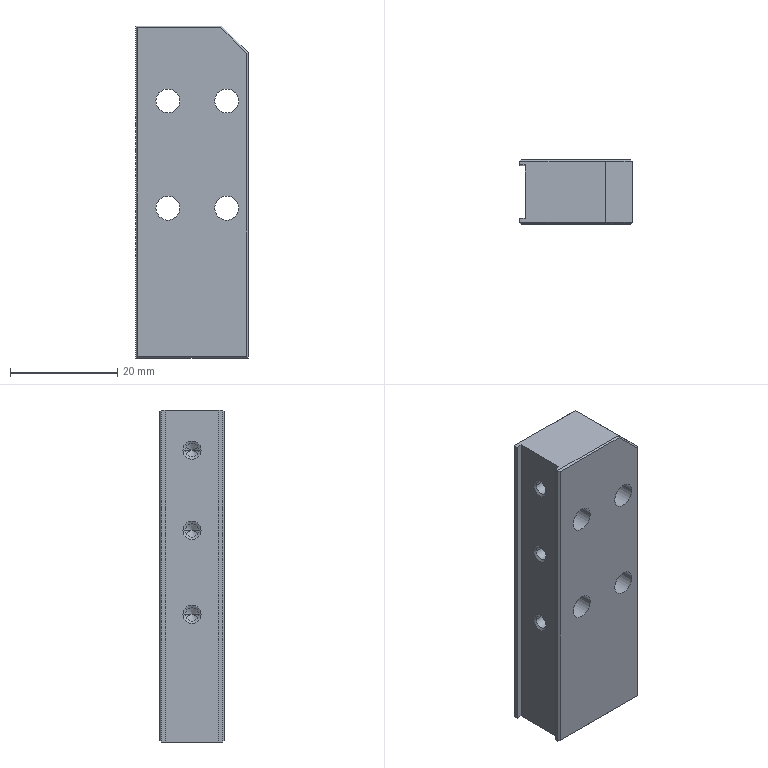Part | NX | 1 solid | 97 faces | box 21 x 12 x 62 mm | volume 13764 mm3 | cylinder 40 | cone 36 | plane 21 | commonest cylinder face diameters 2.5 x32 4.5 x8